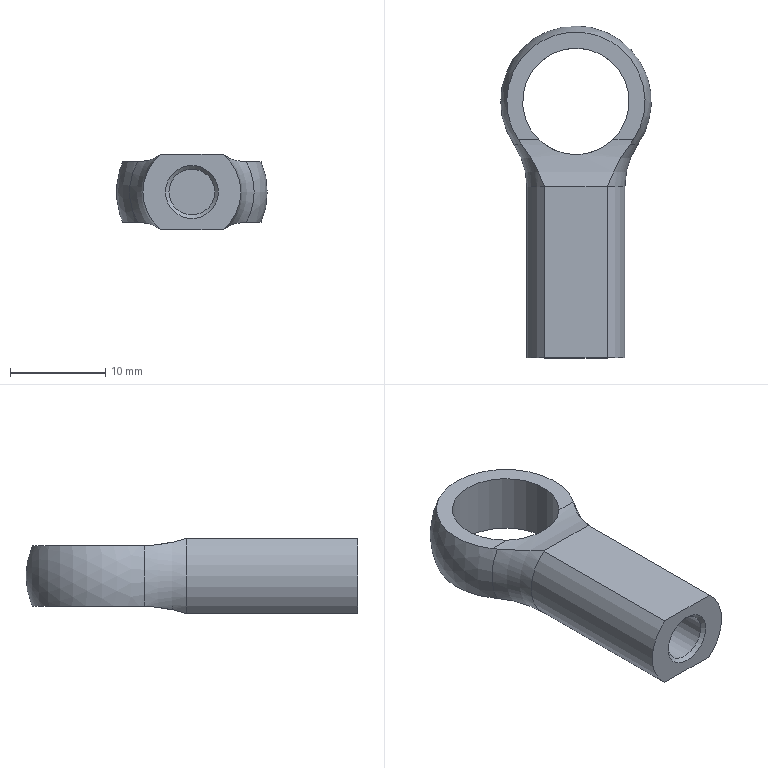Part | NX | features 2458K311 2 | 1 solid | 16 faces | box 15.875 x 34.925 x 7.925 mm | volume 1781 mm3 | plane 6 | cylinder 6 | torus 2 | cone 1 | sphere 1 | commonest cylinder face diameters 10.312 x2 31.75 x2 4.826 x1 11.211 x1
STEP:
#1=CARTESIAN_POINT('',(-5.722,9.799,3.181));
#2=VERTEX_POINT('',#1);
#3=CARTESIAN_POINT('',(-5.722,9.799,-3.181));
#4=VERTEX_POINT('',#3);
#5=CARTESIAN_POINT('',(0.,9.799,0.));
#6=DIRECTION('',(0.,-1.,0.));
#7=DIRECTION('',(1.,0.,0.));
#8=AXIS2_PLACEMENT_3D('',#5,#6,#7);
#9=CIRCLE('',#8,6.547);
#10=EDGE_CURVE('',#2,#4,#9,.T.);
#11=ORIENTED_EDGE('',*,*,#10,.T.);
#12=CARTESIAN_POINT('',(-3.299,5.311,-3.962));
#13=VERTEX_POINT('',#12);
#14=CARTESIAN_POINT('',(-5.722,9.799,-3.181));
#15=CARTESIAN_POINT('',(-4.632,8.437,-3.22));
#16=CARTESIAN_POINT('',(-3.908,6.861,-3.455));
#17=CARTESIAN_POINT('',(-3.299,5.311,-3.962));
#18=B_SPLINE_CURVE_WITH_KNOTS('',3,(#14,#15,#16,#17),.UNSPECIFIED.,.F.,.F.,(4,4),(0.,0.005166),.UNSPECIFIED.);
#19=EDGE_CURVE('',#4,#13,#18,.T.);
#20=ORIENTED_EDGE('',*,*,#19,.T.);
#21=CARTESIAN_POINT('',(-3.299,5.311,3.962));
#22=VERTEX_POINT('',#21);
#23=CARTESIAN_POINT('',(0.,5.311,0.));
#24=DIRECTION('',(0.,1.,0.));
#25=DIRECTION('',(-1.,0.,0.));
#26=AXIS2_PLACEMENT_3D('',#23,#24,#25);
#27=CIRCLE('',#26,5.156);
#28=EDGE_CURVE('',#13,#22,#27,.T.);
#29=ORIENTED_EDGE('',*,*,#28,.T.);
#30=CARTESIAN_POINT('',(-3.299,5.311,3.962));
#31=CARTESIAN_POINT('',(-3.909,6.861,3.455));
#32=CARTESIAN_POINT('',(-4.63,8.435,3.22));
#33=CARTESIAN_POINT('',(-5.722,9.799,3.181));
#34=B_SPLINE_CURVE_WITH_KNOTS('',3,(#30,#31,#32,#33),.UNSPECIFIED.,.F.,.F.,(4,4),(0.,0.005164),.UNSPECIFIED.);
#35=EDGE_CURVE('',#22,#2,#34,.T.);
#36=ORIENTED_EDGE('',*,*,#35,.T.);
#37=EDGE_LOOP('',(#11,#20,#29,#36));
#38=FACE_BOUND('',#37,.T.);
#39=CARTESIAN_POINT('',(0.,5.311,0.));
#40=DIRECTION('',(0.,-1.,0.));
#41=DIRECTION('',(1.,0.,0.));
#42=AXIS2_PLACEMENT_3D('',#39,#40,#41);
#43=TOROIDAL_SURFACE('',#42,13.094,7.938);
#44=ADVANCED_FACE('',(#38),#43,.F.);
#45=CARTESIAN_POINT('',(2.788,-12.7,0.));
#46=VERTEX_POINT('',#45);
#47=CARTESIAN_POINT('',(0.,-12.7,0.));
#48=DIRECTION('',(0.,-1.,0.));
#49=DIRECTION('',(1.,0.,0.));
#50=AXIS2_PLACEMENT_3D('',#47,#48,#49);
#51=CIRCLE('',#50,2.788);
#52=EDGE_CURVE('',#46,#46,#51,.T.);
#53=ORIENTED_EDGE('',*,*,#52,.F.);
#54=EDGE_LOOP('',(#53));
#55=FACE_BOUND('',#54,.T.);
#56=CARTESIAN_POINT('',(-3.299,-12.7,-3.962));
#57=VERTEX_POINT('',#56);
#58=CARTESIAN_POINT('',(3.299,-12.7,-3.962));
#59=VERTEX_POINT('',#58);
#60=CARTESIAN_POINT('',(-3.962,-12.7,-3.962));
#61=DIRECTION('',(1.,0.,0.));
#62=VECTOR('',#61,1000.);
#63=LINE('',#60,#62);
#64=EDGE_CURVE('',#57,#59,#63,.T.);
#65=ORIENTED_EDGE('',*,*,#64,.T.);
#66=CARTESIAN_POINT('',(3.299,-12.7,3.962));
#67=VERTEX_POINT('',#66);
#68=CARTESIAN_POINT('',(0.,-12.7,0.));
#69=DIRECTION('',(0.,1.,0.));
#70=DIRECTION('',(-1.,0.,0.));
#71=AXIS2_PLACEMENT_3D('',#68,#69,#70);
#72=CIRCLE('',#71,5.156);
#73=EDGE_CURVE('',#67,#59,#72,.T.);
#74=ORIENTED_EDGE('',*,*,#73,.F.);
#75=CARTESIAN_POINT('',(-3.299,-12.7,3.962));
#76=VERTEX_POINT('',#75);
#77=CARTESIAN_POINT('',(-3.962,-12.7,3.962));
#78=DIRECTION('',(-1.,0.,0.));
#79=VECTOR('',#78,1000.);
#80=LINE('',#77,#79);
#81=EDGE_CURVE('',#67,#76,#80,.T.);
#82=ORIENTED_EDGE('',*,*,#81,.T.);
#83=CARTESIAN_POINT('',(0.,-12.7,0.));
#84=DIRECTION('',(0.,1.,0.));
#85=DIRECTION('',(-1.,0.,0.));
#86=AXIS2_PLACEMENT_3D('',#83,#84,#85);
#87=CIRCLE('',#86,5.156);
#88=EDGE_CURVE('',#57,#76,#87,.T.);
#89=ORIENTED_EDGE('',*,*,#88,.F.);
#90=EDGE_LOOP('',(#65,#74,#82,#89));
#91=FACE_BOUND('',#90,.T.);
#92=CARTESIAN_POINT('',(5.156,-12.7,0.));
#93=DIRECTION('',(0.,1.,0.));
#94=DIRECTION('',(-1.,0.,0.));
#95=AXIS2_PLACEMENT_3D('',#92,#93,#94);
#96=PLANE('',#95);
#97=ADVANCED_FACE('',(#55,#91),#96,.F.);
#98=CARTESIAN_POINT('',(-3.299,22.225,-3.962));
#99=DIRECTION('',(0.,1.,0.));
#100=VECTOR('',#99,1000.);
#101=LINE('',#98,#100);
#102=EDGE_CURVE('',#57,#13,#101,.T.);
#103=ORIENTED_EDGE('',*,*,#102,.F.);
#104=ORIENTED_EDGE('',*,*,#88,.T.);
#105=CARTESIAN_POINT('',(-3.299,22.225,3.962));
#106=DIRECTION('',(0.,1.,0.));
#107=VECTOR('',#106,1000.);
#108=LINE('',#105,#107);
#109=EDGE_CURVE('',#22,#76,#108,.F.);
#110=ORIENTED_EDGE('',*,*,#109,.F.);
#111=ORIENTED_EDGE('',*,*,#28,.F.);
#112=EDGE_LOOP('',(#103,#104,#110,#111));
#113=FACE_BOUND('',#112,.T.);
#114=CARTESIAN_POINT('',(0.,22.225,0.));
#115=DIRECTION('',(0.,1.,0.));
#116=DIRECTION('',(-1.,0.,0.));
#117=AXIS2_PLACEMENT_3D('',#114,#115,#116);
#118=CYLINDRICAL_SURFACE('',#117,5.156);
#119=ADVANCED_FACE('',(#113),#118,.T.);
#120=CARTESIAN_POINT('',(3.299,5.311,-3.962));
#121=VERTEX_POINT('',#120);
#122=CARTESIAN_POINT('',(3.299,22.225,-3.962));
#123=DIRECTION('',(0.,1.,0.));
#124=VECTOR('',#123,1000.);
#125=LINE('',#122,#124);
#126=EDGE_CURVE('',#121,#59,#125,.F.);
#127=ORIENTED_EDGE('',*,*,#126,.F.);
#128=CARTESIAN_POINT('',(3.299,5.311,3.962));
#129=VERTEX_POINT('',#128);
#130=CARTESIAN_POINT('',(0.,5.311,0.));
#131=DIRECTION('',(0.,1.,0.));
#132=DIRECTION('',(-1.,0.,0.));
#133=AXIS2_PLACEMENT_3D('',#130,#131,#132);
#134=CIRCLE('',#133,5.156);
#135=EDGE_CURVE('',#129,#121,#134,.T.);
#136=ORIENTED_EDGE('',*,*,#135,.F.);
#137=CARTESIAN_POINT('',(3.299,22.225,3.962));
#138=DIRECTION('',(0.,1.,0.));
#139=VECTOR('',#138,1000.);
#140=LINE('',#137,#139);
#141=EDGE_CURVE('',#67,#129,#140,.T.);
#142=ORIENTED_EDGE('',*,*,#141,.F.);
#143=ORIENTED_EDGE('',*,*,#73,.T.);
#144=EDGE_LOOP('',(#127,#136,#142,#143));
#145=FACE_BOUND('',#144,.T.);
#146=CARTESIAN_POINT('',(0.,22.225,0.));
#147=DIRECTION('',(0.,1.,0.));
#148=DIRECTION('',(-1.,0.,0.));
#149=AXIS2_PLACEMENT_3D('',#146,#147,#148);
#150=CYLINDRICAL_SURFACE('',#149,5.156);
#151=ADVANCED_FACE('',(#145),#150,.T.);
#152=ORIENTED_EDGE('',*,*,#141,.T.);
#153=CARTESIAN_POINT('',(0.,5.311,3.962));
#154=DIRECTION('',(-1.,0.,0.));
#155=VECTOR('',#154,1000.);
#156=LINE('',#153,#155);
#157=EDGE_CURVE('',#129,#22,#156,.T.);
#158=ORIENTED_EDGE('',*,*,#157,.T.);
#159=ORIENTED_EDGE('',*,*,#109,.T.);
#160=ORIENTED_EDGE('',*,*,#81,.F.);
#161=EDGE_LOOP('',(#152,#158,#159,#160));
#162=FACE_BOUND('',#161,.T.);
#163=CARTESIAN_POINT('',(-3.962,5.311,3.962));
#164=DIRECTION('',(0.,0.,1.));
#165=DIRECTION('',(1.,0.,0.));
#166=AXIS2_PLACEMENT_3D('',#163,#164,#165);
#167=PLANE('',#166);
#168=ADVANCED_FACE('',(#162),#167,.T.);
#169=ORIENTED_EDGE('',*,*,#102,.T.);
#170=CARTESIAN_POINT('',(0.,5.311,-3.962));
#171=DIRECTION('',(1.,0.,0.));
#172=VECTOR('',#171,1000.);
#173=LINE('',#170,#172);
#174=EDGE_CURVE('',#13,#121,#173,.T.);
#175=ORIENTED_EDGE('',*,*,#174,.T.);
#176=ORIENTED_EDGE('',*,*,#126,.T.);
#177=ORIENTED_EDGE('',*,*,#64,.F.);
#178=EDGE_LOOP('',(#169,#175,#176,#177));
#179=FACE_BOUND('',#178,.T.);
#180=CARTESIAN_POINT('',(-3.962,5.311,-3.962));
#181=DIRECTION('',(0.,0.,-1.));
#182=DIRECTION('',(-1.,0.,0.));
#183=AXIS2_PLACEMENT_3D('',#180,#181,#182);
#184=PLANE('',#183);
#185=ADVANCED_FACE('',(#179),#184,.T.);
#186=CARTESIAN_POINT('',(2.413,-12.325,0.));
#187=VERTEX_POINT('',#186);
#188=CARTESIAN_POINT('',(0.,-12.325,0.));
#189=DIRECTION('',(0.,-1.,0.));
#190=DIRECTION('',(1.,0.,0.));
#191=AXIS2_PLACEMENT_3D('',#188,#189,#190);
#192=CIRCLE('',#191,2.413);
#193=EDGE_CURVE('',#187,#187,#192,.F.);
#194=ORIENTED_EDGE('',*,*,#193,.T.);
#195=EDGE_LOOP('',(#194));
#196=FACE_BOUND('',#195,.T.);
#197=ORIENTED_EDGE('',*,*,#52,.T.);
#198=EDGE_LOOP('',(#197));
#199=FACE_BOUND('',#198,.T.);
#200=CARTESIAN_POINT('',(0.,-12.7,0.));
#201=DIRECTION('',(0.,-1.,0.));
#202=DIRECTION('',(1.,0.,0.));
#203=AXIS2_PLACEMENT_3D('',#200,#201,#202);
#204=CONICAL_SURFACE('',#203,2.788,0.7854);
#205=ADVANCED_FACE('',(#196,#199),#204,.F.);
#206=CARTESIAN_POINT('',(2.413,0.,0.));
#207=VERTEX_POINT('',#206);
#208=CARTESIAN_POINT('',(0.,0.,0.));
#209=DIRECTION('',(0.,-1.,0.));
#210=DIRECTION('',(1.,0.,0.));
#211=AXIS2_PLACEMENT_3D('',#208,#209,#210);
#212=CIRCLE('',#211,2.413);
#213=EDGE_CURVE('',#207,#207,#212,.T.);
#214=ORIENTED_EDGE('',*,*,#213,.F.);
#215=EDGE_LOOP('',(#214));
#216=FACE_BOUND('',#215,.T.);
#217=ORIENTED_EDGE('',*,*,#193,.F.);
#218=EDGE_LOOP('',(#217));
#219=FACE_BOUND('',#218,.T.);
#220=CARTESIAN_POINT('',(0.,0.,0.));
#221=DIRECTION('',(0.,-1.,0.));
#222=DIRECTION('',(1.,0.,0.));
#223=AXIS2_PLACEMENT_3D('',#220,#221,#222);
#224=CYLINDRICAL_SURFACE('',#223,2.413);
#225=ADVANCED_FACE('',(#216,#219),#224,.F.);
#226=ORIENTED_EDGE('',*,*,#213,.T.);
#227=EDGE_LOOP('',(#226));
#228=FACE_BOUND('',#227,.T.);
#229=CARTESIAN_POINT('',(2.413,0.,0.));
#230=DIRECTION('',(0.,1.,0.));
#231=DIRECTION('',(-1.,0.,0.));
#232=AXIS2_PLACEMENT_3D('',#229,#230,#231);
#233=PLANE('',#232);
#234=ADVANCED_FACE('',(#228),#233,.F.);
#235=ORIENTED_EDGE('',*,*,#135,.T.);
#236=CARTESIAN_POINT('',(5.722,9.799,-3.181));
#237=VERTEX_POINT('',#236);
#238=CARTESIAN_POINT('',(3.299,5.311,-3.962));
#239=CARTESIAN_POINT('',(3.909,6.861,-3.455));
#240=CARTESIAN_POINT('',(4.63,8.435,-3.22));
#241=CARTESIAN_POINT('',(5.722,9.799,-3.181));
#242=B_SPLINE_CURVE_WITH_KNOTS('',3,(#238,#239,#240,#241),.UNSPECIFIED.,.F.,.F.,(4,4),(0.,0.005164),.UNSPECIFIED.);
#243=EDGE_CURVE('',#121,#237,#242,.T.);
#244=ORIENTED_EDGE('',*,*,#243,.T.);
#245=CARTESIAN_POINT('',(5.722,9.799,3.181));
#246=VERTEX_POINT('',#245);
#247=CARTESIAN_POINT('',(0.,9.799,0.));
#248=DIRECTION('',(0.,-1.,0.));
#249=DIRECTION('',(1.,0.,0.));
#250=AXIS2_PLACEMENT_3D('',#247,#248,#249);
#251=CIRCLE('',#250,6.547);
#252=EDGE_CURVE('',#237,#246,#251,.T.);
#253=ORIENTED_EDGE('',*,*,#252,.T.);
#254=CARTESIAN_POINT('',(5.722,9.799,3.181));
#255=CARTESIAN_POINT('',(4.632,8.437,3.22));
#256=CARTESIAN_POINT('',(3.908,6.861,3.455));
#257=CARTESIAN_POINT('',(3.299,5.311,3.962));
#258=B_SPLINE_CURVE_WITH_KNOTS('',3,(#254,#255,#256,#257),.UNSPECIFIED.,.F.,.F.,(4,4),(0.,0.005166),.UNSPECIFIED.);
#259=EDGE_CURVE('',#246,#129,#258,.T.);
#260=ORIENTED_EDGE('',*,*,#259,.T.);
#261=EDGE_LOOP('',(#235,#244,#253,#260));
#262=FACE_BOUND('',#261,.T.);
#263=CARTESIAN_POINT('',(0.,5.311,0.));
#264=DIRECTION('',(0.,-1.,0.));
#265=DIRECTION('',(1.,0.,0.));
#266=AXIS2_PLACEMENT_3D('',#263,#264,#265);
#267=TOROIDAL_SURFACE('',#266,13.094,7.938);
#268=ADVANCED_FACE('',(#262),#267,.F.);
#269=CARTESIAN_POINT('',(-6.051,10.249,-3.175));
#270=VERTEX_POINT('',#269);
#271=CARTESIAN_POINT('',(6.051,10.249,-3.175));
#272=VERTEX_POINT('',#271);
#273=CARTESIAN_POINT('',(0.,14.287,-3.175));
#274=DIRECTION('',(0.,0.,1.));
#275=DIRECTION('',(0.,-1.,0.));
#276=AXIS2_PLACEMENT_3D('',#273,#274,#275);
#277=CIRCLE('',#276,7.275);
#278=EDGE_CURVE('',#270,#272,#277,.F.);
#279=ORIENTED_EDGE('',*,*,#278,.F.);
#280=CARTESIAN_POINT('',(-6.051,10.249,-3.175));
#281=CARTESIAN_POINT('',(-5.948,10.094,-3.175));
#282=CARTESIAN_POINT('',(-5.838,9.945,-3.177));
#283=CARTESIAN_POINT('',(-5.722,9.799,-3.181));
#284=B_SPLINE_CURVE_WITH_KNOTS('',3,(#280,#281,#282,#283),.UNSPECIFIED.,.F.,.F.,(4,4),(0.,0.0005571),.UNSPECIFIED.);
#285=EDGE_CURVE('',#270,#4,#284,.T.);
#286=ORIENTED_EDGE('',*,*,#285,.T.);
#287=ORIENTED_EDGE('',*,*,#10,.F.);
#288=CARTESIAN_POINT('',(-6.051,10.249,3.175));
#289=VERTEX_POINT('',#288);
#290=CARTESIAN_POINT('',(-5.722,9.799,3.181));
#291=CARTESIAN_POINT('',(-5.838,9.945,3.177));
#292=CARTESIAN_POINT('',(-5.948,10.094,3.175));
#293=CARTESIAN_POINT('',(-6.051,10.249,3.175));
#294=B_SPLINE_CURVE_WITH_KNOTS('',3,(#290,#291,#292,#293),.UNSPECIFIED.,.F.,.F.,(4,4),(0.,0.0005571),.UNSPECIFIED.);
#295=EDGE_CURVE('',#2,#289,#294,.T.);
#296=ORIENTED_EDGE('',*,*,#295,.T.);
#297=CARTESIAN_POINT('',(6.051,10.249,3.175));
#298=VERTEX_POINT('',#297);
#299=CARTESIAN_POINT('',(0.,14.287,3.175));
#300=DIRECTION('',(0.,0.,-1.));
#301=DIRECTION('',(0.,1.,0.));
#302=AXIS2_PLACEMENT_3D('',#299,#300,#301);
#303=CIRCLE('',#302,7.275);
#304=EDGE_CURVE('',#298,#289,#303,.F.);
#305=ORIENTED_EDGE('',*,*,#304,.F.);
#306=CARTESIAN_POINT('',(6.051,10.249,3.175));
#307=CARTESIAN_POINT('',(5.948,10.094,3.175));
#308=CARTESIAN_POINT('',(5.838,9.945,3.177));
#309=CARTESIAN_POINT('',(5.722,9.799,3.181));
#310=B_SPLINE_CURVE_WITH_KNOTS('',3,(#306,#307,#308,#309),.UNSPECIFIED.,.F.,.F.,(4,4),(0.,0.0005571),.UNSPECIFIED.);
#311=EDGE_CURVE('',#298,#246,#310,.T.);
#312=ORIENTED_EDGE('',*,*,#311,.T.);
#313=ORIENTED_EDGE('',*,*,#252,.F.);
#314=CARTESIAN_POINT('',(5.722,9.799,-3.181));
#315=CARTESIAN_POINT('',(5.838,9.945,-3.177));
#316=CARTESIAN_POINT('',(5.948,10.094,-3.175));
#317=CARTESIAN_POINT('',(6.051,10.249,-3.175));
#318=B_SPLINE_CURVE_WITH_KNOTS('',3,(#314,#315,#316,#317),.UNSPECIFIED.,.F.,.F.,(4,4),(0.,0.0005571),.UNSPECIFIED.);
#319=EDGE_CURVE('',#237,#272,#318,.T.);
#320=ORIENTED_EDGE('',*,*,#319,.T.);
#321=EDGE_LOOP('',(#279,#286,#287,#296,#305,#312,#313,#320));
#322=FACE_BOUND('',#321,.T.);
#323=CARTESIAN_POINT('',(0.,14.287,0.));
#324=DIRECTION('',(0.,-1.,0.));
#325=DIRECTION('',(1.,0.,0.));
#326=AXIS2_PLACEMENT_3D('',#323,#324,#325);
#327=SPHERICAL_SURFACE('',#326,7.938);
#328=ADVANCED_FACE('',(#322),#327,.T.);
#329=CARTESIAN_POINT('',(-3.887,10.249,3.175));
#330=VERTEX_POINT('',#329);
#331=CARTESIAN_POINT('',(-7.938,10.249,3.175));
#332=DIRECTION('',(-1.,0.,0.));
#333=VECTOR('',#332,1000.);
#334=LINE('',#331,#333);
#335=EDGE_CURVE('',#289,#330,#334,.F.);
#336=ORIENTED_EDGE('',*,*,#335,.T.);
#337=CARTESIAN_POINT('',(3.887,10.249,3.175));
#338=VERTEX_POINT('',#337);
#339=CARTESIAN_POINT('',(0.,14.287,3.175));
#340=DIRECTION('',(0.,0.,-1.));
#341=DIRECTION('',(0.,1.,0.));
#342=AXIS2_PLACEMENT_3D('',#339,#340,#341);
#343=CIRCLE('',#342,5.605);
#344=EDGE_CURVE('',#330,#338,#343,.T.);
#345=ORIENTED_EDGE('',*,*,#344,.T.);
#346=CARTESIAN_POINT('',(-7.938,10.249,3.175));
#347=DIRECTION('',(-1.,0.,0.));
#348=VECTOR('',#347,1000.);
#349=LINE('',#346,#348);
#350=EDGE_CURVE('',#338,#298,#349,.F.);
#351=ORIENTED_EDGE('',*,*,#350,.T.);
#352=ORIENTED_EDGE('',*,*,#304,.T.);
#353=EDGE_LOOP('',(#336,#345,#351,#352));
#354=FACE_BOUND('',#353,.T.);
#355=CARTESIAN_POINT('',(-7.938,22.225,3.175));
#356=DIRECTION('',(0.,0.,-1.));
#357=DIRECTION('',(0.,1.,0.));
#358=AXIS2_PLACEMENT_3D('',#355,#356,#357);
#359=PLANE('',#358);
#360=ADVANCED_FACE('',(#354),#359,.F.);
#361=CARTESIAN_POINT('',(3.887,10.249,-3.175));
#362=VERTEX_POINT('',#361);
#363=CARTESIAN_POINT('',(-7.938,10.249,-3.175));
#364=DIRECTION('',(1.,0.,0.));
#365=VECTOR('',#364,1000.);
#366=LINE('',#363,#365);
#367=EDGE_CURVE('',#272,#362,#366,.F.);
#368=ORIENTED_EDGE('',*,*,#367,.T.);
#369=CARTESIAN_POINT('',(-3.887,10.249,-3.175));
#370=VERTEX_POINT('',#369);
#371=CARTESIAN_POINT('',(0.,14.287,-3.175));
#372=DIRECTION('',(0.,0.,1.));
#373=DIRECTION('',(0.,-1.,0.));
#374=AXIS2_PLACEMENT_3D('',#371,#372,#373);
#375=CIRCLE('',#374,5.605);
#376=EDGE_CURVE('',#362,#370,#375,.T.);
#377=ORIENTED_EDGE('',*,*,#376,.T.);
#378=CARTESIAN_POINT('',(-7.938,10.249,-3.175));
#379=DIRECTION('',(1.,0.,0.));
#380=VECTOR('',#379,1000.);
#381=LINE('',#378,#380);
#382=EDGE_CURVE('',#370,#270,#381,.F.);
#383=ORIENTED_EDGE('',*,*,#382,.T.);
#384=ORIENTED_EDGE('',*,*,#278,.T.);
#385=EDGE_LOOP('',(#368,#377,#383,#384));
#386=FACE_BOUND('',#385,.T.);
#387=CARTESIAN_POINT('',(-7.938,22.225,-3.175));
#388=DIRECTION('',(0.,0.,1.));
#389=DIRECTION('',(0.,-1.,0.));
#390=AXIS2_PLACEMENT_3D('',#387,#388,#389);
#391=PLANE('',#390);
#392=ADVANCED_FACE('',(#386),#391,.F.);
#393=ORIENTED_EDGE('',*,*,#350,.F.);
#394=CARTESIAN_POINT('',(3.887,10.249,3.175));
#395=CARTESIAN_POINT('',(2.846,9.247,3.175));
#396=CARTESIAN_POINT('',(0.003795,8.117,3.33));
#397=CARTESIAN_POINT('',(-2.846,9.247,3.175));
#398=CARTESIAN_POINT('',(-3.887,10.249,3.175));
#399=B_SPLINE_CURVE_WITH_KNOTS('',3,(#394,#395,#396,#397,#398),.UNSPECIFIED.,.F.,.F.,(4,1,4),(0.,0.004272,0.008545),.UNSPECIFIED.);
#400=EDGE_CURVE('',#338,#330,#399,.T.);
#401=ORIENTED_EDGE('',*,*,#400,.T.);
#402=ORIENTED_EDGE('',*,*,#335,.F.);
#403=ORIENTED_EDGE('',*,*,#295,.F.);
#404=ORIENTED_EDGE('',*,*,#35,.F.);
#405=ORIENTED_EDGE('',*,*,#157,.F.);
#406=ORIENTED_EDGE('',*,*,#259,.F.);
#407=ORIENTED_EDGE('',*,*,#311,.F.);
#408=EDGE_LOOP('',(#393,#401,#402,#403,#404,#405,#406,#407));
#409=FACE_BOUND('',#408,.T.);
#410=CARTESIAN_POINT('',(-7.938,10.249,19.05));
#411=DIRECTION('',(-1.,0.,0.));
#412=DIRECTION('',(0.,0.,1.));
#413=AXIS2_PLACEMENT_3D('',#410,#411,#412);
#414=CYLINDRICAL_SURFACE('',#413,15.875);
#415=ADVANCED_FACE('',(#409),#414,.F.);
#416=ORIENTED_EDGE('',*,*,#382,.F.);
#417=CARTESIAN_POINT('',(-3.887,10.249,-3.175));
#418=CARTESIAN_POINT('',(-2.846,9.247,-3.175));
#419=CARTESIAN_POINT('',(-0.003795,8.117,-3.33));
#420=CARTESIAN_POINT('',(2.846,9.247,-3.175));
#421=CARTESIAN_POINT('',(3.887,10.249,-3.175));
#422=B_SPLINE_CURVE_WITH_KNOTS('',3,(#417,#418,#419,#420,#421),.UNSPECIFIED.,.F.,.F.,(4,1,4),(0.,0.004272,0.008545),.UNSPECIFIED.);
#423=EDGE_CURVE('',#370,#362,#422,.T.);
#424=ORIENTED_EDGE('',*,*,#423,.T.);
#425=ORIENTED_EDGE('',*,*,#367,.F.);
#426=ORIENTED_EDGE('',*,*,#319,.F.);
#427=ORIENTED_EDGE('',*,*,#243,.F.);
#428=ORIENTED_EDGE('',*,*,#174,.F.);
#429=ORIENTED_EDGE('',*,*,#19,.F.);
#430=ORIENTED_EDGE('',*,*,#285,.F.);
#431=EDGE_LOOP('',(#416,#424,#425,#426,#427,#428,#429,#430));
#432=FACE_BOUND('',#431,.T.);
#433=CARTESIAN_POINT('',(-7.938,10.249,-19.05));
#434=DIRECTION('',(1.,0.,0.));
#435=DIRECTION('',(0.,0.,-1.));
#436=AXIS2_PLACEMENT_3D('',#433,#434,#435);
#437=CYLINDRICAL_SURFACE('',#436,15.875);
#438=ADVANCED_FACE('',(#432),#437,.F.);
#439=ORIENTED_EDGE('',*,*,#423,.F.);
#440=ORIENTED_EDGE('',*,*,#376,.F.);
#441=EDGE_LOOP('',(#439,#440));
#442=FACE_BOUND('',#441,.T.);
#443=ORIENTED_EDGE('',*,*,#400,.F.);
#444=ORIENTED_EDGE('',*,*,#344,.F.);
#445=EDGE_LOOP('',(#443,#444));
#446=FACE_BOUND('',#445,.T.);
#447=CARTESIAN_POINT('',(0.,14.287,-4.706));
#448=DIRECTION('',(0.,0.,1.));
#449=DIRECTION('',(1.,0.,0.));
#450=AXIS2_PLACEMENT_3D('',#447,#448,#449);
#451=CYLINDRICAL_SURFACE('',#450,5.605);
#452=ADVANCED_FACE('',(#442,#446),#451,.F.);
#453=CLOSED_SHELL('',(#44,#97,#119,#151,#168,#185,#205,#225,#234,#268,#328,#360,#392,#415,#438,#452));
#454=MANIFOLD_SOLID_BREP('',#453);
#455=(LENGTH_UNIT()NAMED_UNIT(*)SI_UNIT(.MILLI.,.METRE.));
#456=UNCERTAINTY_MEASURE_WITH_UNIT(LENGTH_MEASURE(0.0508),#455,'','');
#457=(NAMED_UNIT(*)PLANE_ANGLE_UNIT()SI_UNIT($,.RADIAN.));
#458=(NAMED_UNIT(*)SI_UNIT($,.STERADIAN.)SOLID_ANGLE_UNIT());
#459=(GEOMETRIC_REPRESENTATION_CONTEXT(3)GLOBAL_UNCERTAINTY_ASSIGNED_CONTEXT((#456))GLOBAL_UNIT_ASSIGNED_CONTEXT((#455,#457,#458))REPRESENTATION_CONTEXT('',''));
#460=ADVANCED_BREP_SHAPE_REPRESENTATION('',(#454),#459);